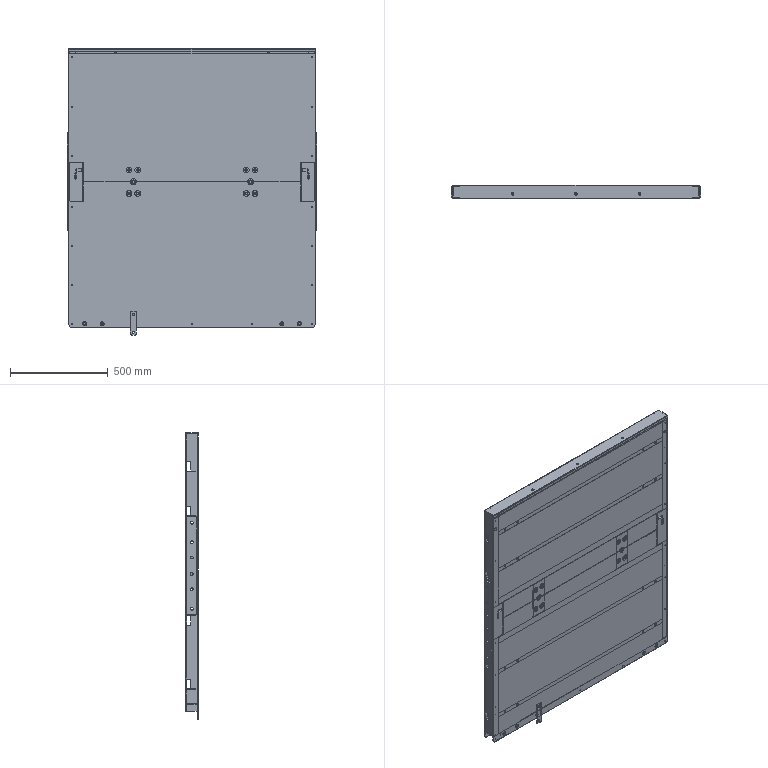Part | SolidWorks | 58 solids | 1698 faces | box 1280 x 70 x 1465 mm | volume 13190412 mm3 | plane 1006 | cylinder 590 | cone 102 | commonest cylinder face diameters 10 x90 14.5 x88 11 x84 0.4 x36 5 x34 20 x32